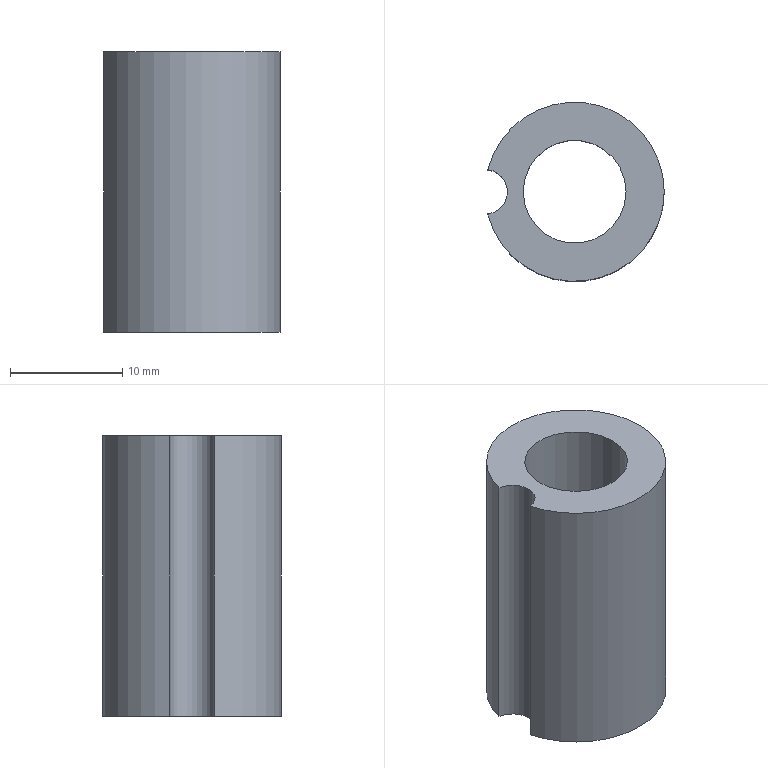Part | NX | features solid 2 | 1 solid | 7 faces | box 15.75 x 16 x 25 mm | volume 2932 mm3 | cylinder 4 | plane 3 | commonest cylinder face diameters 4 x1 9.18 x1 10.3 x1 16 x1
STEP:
#1=CARTESIAN_POINT('',(507.846,-160.118,-37.396));
#2=VERTEX_POINT('',#1);
#3=CARTESIAN_POINT('',(507.846,-164.087,-37.396));
#4=VERTEX_POINT('',#3);
#5=CARTESIAN_POINT('',(507.596,-162.103,-37.396));
#6=DIRECTION('',(0.,0.,-1.));
#7=DIRECTION('',(-1.,0.,0.));
#8=AXIS2_PLACEMENT_3D('',#5,#6,#7);
#9=CIRCLE('',#8,2.);
#10=EDGE_CURVE('',#2,#4,#9,.T.);
#11=ORIENTED_EDGE('',*,*,#10,.F.);
#12=CARTESIAN_POINT('',(515.596,-162.103,-37.396));
#13=DIRECTION('',(0.,0.,1.));
#14=DIRECTION('',(1.,0.,0.));
#15=AXIS2_PLACEMENT_3D('',#12,#13,#14);
#16=CIRCLE('',#15,8.);
#17=EDGE_CURVE('',#2,#4,#16,.F.);
#18=ORIENTED_EDGE('',*,*,#17,.T.);
#19=EDGE_LOOP('',(#11,#18));
#20=FACE_BOUND('',#19,.T.);
#21=CARTESIAN_POINT('',(520.746,-162.103,-37.396));
#22=VERTEX_POINT('',#21);
#23=CARTESIAN_POINT('',(515.596,-162.103,-37.396));
#24=DIRECTION('',(0.,0.,1.));
#25=DIRECTION('',(1.,0.,0.));
#26=AXIS2_PLACEMENT_3D('',#23,#24,#25);
#27=CIRCLE('',#26,5.15);
#28=EDGE_CURVE('',#22,#22,#27,.T.);
#29=ORIENTED_EDGE('',*,*,#28,.T.);
#30=EDGE_LOOP('',(#29));
#31=FACE_BOUND('',#30,.T.);
#32=CARTESIAN_POINT('',(515.596,-162.103,-37.396));
#33=DIRECTION('',(0.,0.,-1.));
#34=DIRECTION('',(1.,0.,0.));
#35=AXIS2_PLACEMENT_3D('',#32,#33,#34);
#36=PLANE('',#35);
#37=ADVANCED_FACE('',(#20,#31),#36,.T.);
#38=CARTESIAN_POINT('',(507.846,-160.118,-12.396));
#39=VERTEX_POINT('',#38);
#40=CARTESIAN_POINT('',(507.846,-164.087,-12.396));
#41=VERTEX_POINT('',#40);
#42=CARTESIAN_POINT('',(507.596,-162.103,-12.396));
#43=DIRECTION('',(0.,0.,-1.));
#44=DIRECTION('',(-1.,0.,0.));
#45=AXIS2_PLACEMENT_3D('',#42,#43,#44);
#46=CIRCLE('',#45,2.);
#47=EDGE_CURVE('',#39,#41,#46,.T.);
#48=ORIENTED_EDGE('',*,*,#47,.T.);
#49=CARTESIAN_POINT('',(515.596,-162.103,-12.396));
#50=DIRECTION('',(0.,0.,-1.));
#51=DIRECTION('',(-1.,0.,0.));
#52=AXIS2_PLACEMENT_3D('',#49,#50,#51);
#53=CIRCLE('',#52,8.);
#54=EDGE_CURVE('',#41,#39,#53,.F.);
#55=ORIENTED_EDGE('',*,*,#54,.T.);
#56=EDGE_LOOP('',(#48,#55));
#57=FACE_BOUND('',#56,.T.);
#58=CARTESIAN_POINT('',(520.186,-162.103,-12.396));
#59=VERTEX_POINT('',#58);
#60=CARTESIAN_POINT('',(515.596,-162.103,-12.396));
#61=DIRECTION('',(0.,0.,1.));
#62=DIRECTION('',(1.,0.,0.));
#63=AXIS2_PLACEMENT_3D('',#60,#61,#62);
#64=CIRCLE('',#63,4.59);
#65=EDGE_CURVE('',#59,#59,#64,.T.);
#66=ORIENTED_EDGE('',*,*,#65,.F.);
#67=EDGE_LOOP('',(#66));
#68=FACE_BOUND('',#67,.T.);
#69=CARTESIAN_POINT('',(515.596,-162.103,-12.396));
#70=DIRECTION('',(0.,0.,1.));
#71=DIRECTION('',(-1.,0.,0.));
#72=AXIS2_PLACEMENT_3D('',#69,#70,#71);
#73=PLANE('',#72);
#74=ADVANCED_FACE('',(#57,#68),#73,.T.);
#75=CARTESIAN_POINT('',(507.846,-164.087,-24.896));
#76=DIRECTION('',(0.,0.,1.));
#77=VECTOR('',#76,1000.);
#78=LINE('',#75,#77);
#79=EDGE_CURVE('',#4,#41,#78,.T.);
#80=ORIENTED_EDGE('',*,*,#79,.F.);
#81=ORIENTED_EDGE('',*,*,#17,.F.);
#82=CARTESIAN_POINT('',(507.846,-160.118,-24.896));
#83=DIRECTION('',(0.,0.,1.));
#84=VECTOR('',#83,1000.);
#85=LINE('',#82,#84);
#86=EDGE_CURVE('',#39,#2,#85,.F.);
#87=ORIENTED_EDGE('',*,*,#86,.F.);
#88=ORIENTED_EDGE('',*,*,#54,.F.);
#89=EDGE_LOOP('',(#80,#81,#87,#88));
#90=FACE_BOUND('',#89,.T.);
#91=CARTESIAN_POINT('',(515.596,-162.103,-37.396));
#92=DIRECTION('',(0.,0.,1.));
#93=DIRECTION('',(-1.,0.,0.));
#94=AXIS2_PLACEMENT_3D('',#91,#92,#93);
#95=CYLINDRICAL_SURFACE('',#94,8.);
#96=ADVANCED_FACE('',(#90),#95,.T.);
#97=ORIENTED_EDGE('',*,*,#65,.T.);
#98=EDGE_LOOP('',(#97));
#99=FACE_BOUND('',#98,.T.);
#100=CARTESIAN_POINT('',(520.186,-162.103,-20.396));
#101=VERTEX_POINT('',#100);
#102=CARTESIAN_POINT('',(515.596,-162.103,-20.396));
#103=DIRECTION('',(0.,0.,1.));
#104=DIRECTION('',(1.,0.,0.));
#105=AXIS2_PLACEMENT_3D('',#102,#103,#104);
#106=CIRCLE('',#105,4.59);
#107=EDGE_CURVE('',#101,#101,#106,.F.);
#108=ORIENTED_EDGE('',*,*,#107,.T.);
#109=EDGE_LOOP('',(#108));
#110=FACE_BOUND('',#109,.T.);
#111=CARTESIAN_POINT('',(515.596,-162.103,-20.396));
#112=DIRECTION('',(0.,0.,1.));
#113=DIRECTION('',(-1.,0.,0.));
#114=AXIS2_PLACEMENT_3D('',#111,#112,#113);
#115=CYLINDRICAL_SURFACE('',#114,4.59);
#116=ADVANCED_FACE('',(#99,#110),#115,.F.);
#117=ORIENTED_EDGE('',*,*,#86,.T.);
#118=ORIENTED_EDGE('',*,*,#10,.T.);
#119=ORIENTED_EDGE('',*,*,#79,.T.);
#120=ORIENTED_EDGE('',*,*,#47,.F.);
#121=EDGE_LOOP('',(#117,#118,#119,#120));
#122=FACE_BOUND('',#121,.T.);
#123=CARTESIAN_POINT('',(507.596,-162.103,-37.396));
#124=DIRECTION('',(0.,0.,1.));
#125=DIRECTION('',(-1.,0.,0.));
#126=AXIS2_PLACEMENT_3D('',#123,#124,#125);
#127=CYLINDRICAL_SURFACE('',#126,2.);
#128=ADVANCED_FACE('',(#122),#127,.F.);
#129=CARTESIAN_POINT('',(520.746,-162.103,-20.396));
#130=VERTEX_POINT('',#129);
#131=CARTESIAN_POINT('',(515.596,-162.103,-20.396));
#132=DIRECTION('',(0.,0.,1.));
#133=DIRECTION('',(1.,0.,0.));
#134=AXIS2_PLACEMENT_3D('',#131,#132,#133);
#135=CIRCLE('',#134,5.15);
#136=EDGE_CURVE('',#130,#130,#135,.T.);
#137=ORIENTED_EDGE('',*,*,#136,.F.);
#138=EDGE_LOOP('',(#137));
#139=FACE_BOUND('',#138,.T.);
#140=ORIENTED_EDGE('',*,*,#107,.F.);
#141=EDGE_LOOP('',(#140));
#142=FACE_BOUND('',#141,.T.);
#143=CARTESIAN_POINT('',(515.596,-162.103,-20.396));
#144=DIRECTION('',(0.,0.,1.));
#145=DIRECTION('',(1.,0.,0.));
#146=AXIS2_PLACEMENT_3D('',#143,#144,#145);
#147=PLANE('',#146);
#148=ADVANCED_FACE('',(#139,#142),#147,.F.);
#149=ORIENTED_EDGE('',*,*,#136,.T.);
#150=EDGE_LOOP('',(#149));
#151=FACE_BOUND('',#150,.T.);
#152=ORIENTED_EDGE('',*,*,#28,.F.);
#153=EDGE_LOOP('',(#152));
#154=FACE_BOUND('',#153,.T.);
#155=CARTESIAN_POINT('',(515.596,-162.103,-20.396));
#156=DIRECTION('',(0.,0.,-1.));
#157=DIRECTION('',(-1.,0.,0.));
#158=AXIS2_PLACEMENT_3D('',#155,#156,#157);
#159=CYLINDRICAL_SURFACE('',#158,5.15);
#160=ADVANCED_FACE('',(#151,#154),#159,.F.);
#161=CLOSED_SHELL('',(#37,#74,#96,#116,#128,#148,#160));
#162=MANIFOLD_SOLID_BREP('',#161);
#163=(LENGTH_UNIT()NAMED_UNIT(*)SI_UNIT(.MILLI.,.METRE.));
#164=UNCERTAINTY_MEASURE_WITH_UNIT(LENGTH_MEASURE(0.00001),#163,'','');
#165=(NAMED_UNIT(*)PLANE_ANGLE_UNIT()SI_UNIT($,.RADIAN.));
#166=(NAMED_UNIT(*)SI_UNIT($,.STERADIAN.)SOLID_ANGLE_UNIT());
#167=(GEOMETRIC_REPRESENTATION_CONTEXT(3)GLOBAL_UNCERTAINTY_ASSIGNED_CONTEXT((#164))GLOBAL_UNIT_ASSIGNED_CONTEXT((#163,#165,#166))REPRESENTATION_CONTEXT('',''));
#168=ADVANCED_BREP_SHAPE_REPRESENTATION('',(#162),#167);